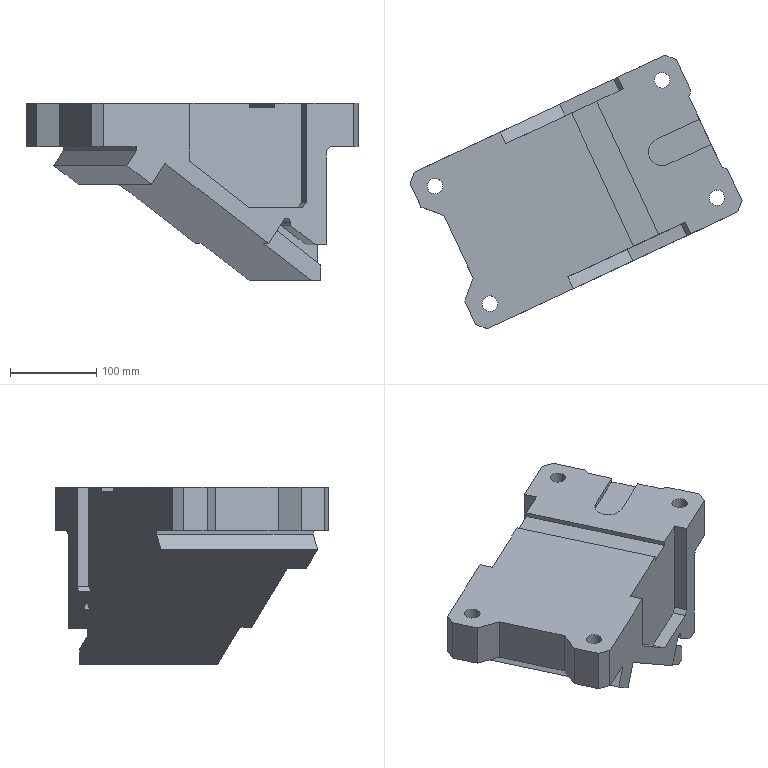Part | NX | features solid 2 | 1 solid | 73 faces | box 384.216 x 316.499 x 205 mm | volume 6626751 mm3 | plane 62 | cylinder 11 | commonest cylinder face diameters 18 x4 26 x4 10 x2 32 x1